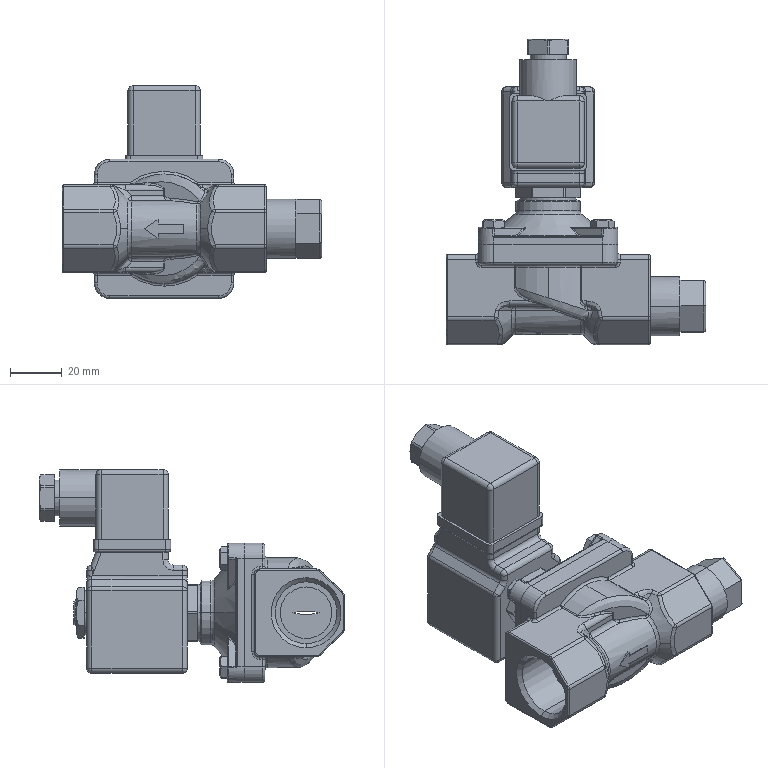Part | SolidWorks | features CompositeCurve 1 | 9 solids | 644 faces | box 100.614 x 118.43 x 82.5 mm | volume 197433 mm3 | cylinder 188 | plane 185 | spline 139 | torus 66 | cone 34 | sphere 32 | commonest cylinder face diameters 4 x60 2 x43 1 x32 25 x9 12 x8 18 x6